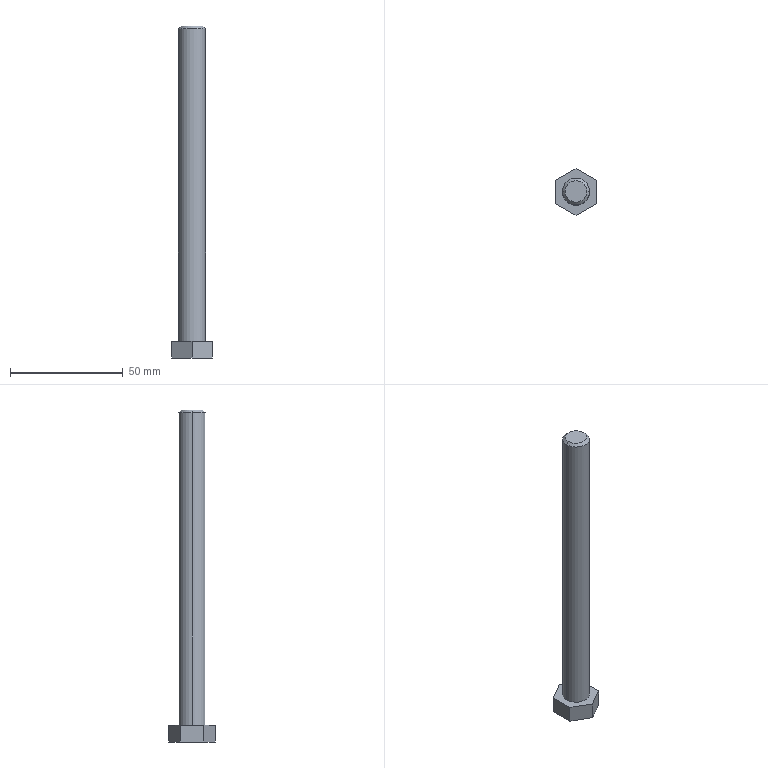Part | SolidWorks | features Chamfer 1, Extrusion 1, ICE 1, RefAxis 1 | 1 solid | 13 faces | box 18 x 20.785 x 147.5 mm | volume 17913 mm3 | plane 9 | cone 2 | cylinder 2 | commonest cylinder face diameters 12 x2
STEP:
#1=CARTESIAN_POINT('',(4.8,0.,147.5));
#2=VERTEX_POINT('',#1);
#3=CARTESIAN_POINT('',(-4.8,0.,147.5));
#4=VERTEX_POINT('',#3);
#5=CARTESIAN_POINT('',(0.,0.,147.5));
#6=DIRECTION('',(0.,0.,1.));
#7=DIRECTION('',(1.,0.,0.));
#8=AXIS2_PLACEMENT_3D('',#5,#6,#7);
#9=CIRCLE('',#8,4.8);
#10=EDGE_CURVE('',#2,#4,#9,.T.);
#11=ORIENTED_EDGE('',*,*,#10,.F.);
#12=CARTESIAN_POINT('',(6.,0.,146.3));
#13=VERTEX_POINT('',#12);
#14=CARTESIAN_POINT('',(4.8,0.,147.5));
#15=DIRECTION('',(0.7071,0.,-0.7071));
#16=VECTOR('',#15,1000.);
#17=LINE('',#14,#16);
#18=EDGE_CURVE('',#2,#13,#17,.T.);
#19=ORIENTED_EDGE('',*,*,#18,.T.);
#20=CARTESIAN_POINT('',(-6.,0.,146.3));
#21=VERTEX_POINT('',#20);
#22=CARTESIAN_POINT('',(0.,0.,146.3));
#23=DIRECTION('',(0.,0.,-1.));
#24=DIRECTION('',(1.,0.,0.));
#25=AXIS2_PLACEMENT_3D('',#22,#23,#24);
#26=CIRCLE('',#25,6.);
#27=EDGE_CURVE('',#21,#13,#26,.T.);
#28=ORIENTED_EDGE('',*,*,#27,.F.);
#29=CARTESIAN_POINT('',(-4.8,0.,147.5));
#30=DIRECTION('',(-0.7071,0.,-0.7071));
#31=VECTOR('',#30,1000.);
#32=LINE('',#29,#31);
#33=EDGE_CURVE('',#4,#21,#32,.T.);
#34=ORIENTED_EDGE('',*,*,#33,.F.);
#35=EDGE_LOOP('',(#11,#19,#28,#34));
#36=FACE_OUTER_BOUND('',#35,.T.);
#37=CARTESIAN_POINT('',(0.,0.,147.5));
#38=DIRECTION('',(0.,0.,-1.));
#39=DIRECTION('',(-1.,0.,0.));
#40=AXIS2_PLACEMENT_3D('',#37,#38,#39);
#41=CONICAL_SURFACE('',#40,4.8,0.7854);
#42=ADVANCED_FACE('',(#36),#41,.T.);
#43=ORIENTED_EDGE('',*,*,#27,.T.);
#44=CARTESIAN_POINT('',(6.,0.,7.5));
#45=VERTEX_POINT('',#44);
#46=CARTESIAN_POINT('',(6.,0.,147.5));
#47=DIRECTION('',(0.,0.,-1.));
#48=VECTOR('',#47,1000.);
#49=LINE('',#46,#48);
#50=EDGE_CURVE('',#13,#45,#49,.T.);
#51=ORIENTED_EDGE('',*,*,#50,.T.);
#52=CARTESIAN_POINT('',(-6.,0.,7.5));
#53=VERTEX_POINT('',#52);
#54=CARTESIAN_POINT('',(0.,0.,7.5));
#55=DIRECTION('',(0.,0.,1.));
#56=DIRECTION('',(1.,0.,0.));
#57=AXIS2_PLACEMENT_3D('',#54,#55,#56);
#58=CIRCLE('',#57,6.);
#59=EDGE_CURVE('',#45,#53,#58,.T.);
#60=ORIENTED_EDGE('',*,*,#59,.T.);
#61=CARTESIAN_POINT('',(-6.,0.,147.5));
#62=DIRECTION('',(0.,0.,-1.));
#63=VECTOR('',#62,1000.);
#64=LINE('',#61,#63);
#65=EDGE_CURVE('',#21,#53,#64,.T.);
#66=ORIENTED_EDGE('',*,*,#65,.F.);
#67=EDGE_LOOP('',(#43,#51,#60,#66));
#68=FACE_OUTER_BOUND('',#67,.T.);
#69=CARTESIAN_POINT('',(0.,0.,147.5));
#70=DIRECTION('',(0.,0.,-1.));
#71=DIRECTION('',(-1.,0.,0.));
#72=AXIS2_PLACEMENT_3D('',#69,#70,#71);
#73=CYLINDRICAL_SURFACE('',#72,6.);
#74=ADVANCED_FACE('',(#68),#73,.T.);
#75=CARTESIAN_POINT('',(9.,-5.196,7.5));
#76=VERTEX_POINT('',#75);
#77=CARTESIAN_POINT('',(9.,5.196,7.5));
#78=VERTEX_POINT('',#77);
#79=CARTESIAN_POINT('',(9.,-5.196,7.5));
#80=DIRECTION('',(0.,1.,0.));
#81=VECTOR('',#80,1000.);
#82=LINE('',#79,#81);
#83=EDGE_CURVE('',#76,#78,#82,.T.);
#84=ORIENTED_EDGE('',*,*,#83,.T.);
#85=CARTESIAN_POINT('',(0.,10.392,7.5));
#86=VERTEX_POINT('',#85);
#87=CARTESIAN_POINT('',(9.,5.196,7.5));
#88=DIRECTION('',(-0.866,0.5,0.));
#89=VECTOR('',#88,1000.);
#90=LINE('',#87,#89);
#91=EDGE_CURVE('',#78,#86,#90,.T.);
#92=ORIENTED_EDGE('',*,*,#91,.T.);
#93=CARTESIAN_POINT('',(-9.,5.196,7.5));
#94=VERTEX_POINT('',#93);
#95=CARTESIAN_POINT('',(0.,10.392,7.5));
#96=DIRECTION('',(-0.866,-0.5,0.));
#97=VECTOR('',#96,1000.);
#98=LINE('',#95,#97);
#99=EDGE_CURVE('',#86,#94,#98,.T.);
#100=ORIENTED_EDGE('',*,*,#99,.T.);
#101=CARTESIAN_POINT('',(-9.,-5.196,7.5));
#102=VERTEX_POINT('',#101);
#103=CARTESIAN_POINT('',(-9.,5.196,7.5));
#104=DIRECTION('',(0.,-1.,0.));
#105=VECTOR('',#104,1000.);
#106=LINE('',#103,#105);
#107=EDGE_CURVE('',#94,#102,#106,.T.);
#108=ORIENTED_EDGE('',*,*,#107,.T.);
#109=CARTESIAN_POINT('',(0.,-10.392,7.5));
#110=VERTEX_POINT('',#109);
#111=CARTESIAN_POINT('',(-9.,-5.196,7.5));
#112=DIRECTION('',(0.866,-0.5,0.));
#113=VECTOR('',#112,1000.);
#114=LINE('',#111,#113);
#115=EDGE_CURVE('',#102,#110,#114,.T.);
#116=ORIENTED_EDGE('',*,*,#115,.T.);
#117=CARTESIAN_POINT('',(0.,-10.392,7.5));
#118=DIRECTION('',(0.866,0.5,0.));
#119=VECTOR('',#118,1000.);
#120=LINE('',#117,#119);
#121=EDGE_CURVE('',#110,#76,#120,.T.);
#122=ORIENTED_EDGE('',*,*,#121,.T.);
#123=EDGE_LOOP('',(#84,#92,#100,#108,#116,#122));
#124=FACE_OUTER_BOUND('',#123,.T.);
#125=CARTESIAN_POINT('',(0.,0.,7.5));
#126=DIRECTION('',(0.,0.,1.));
#127=DIRECTION('',(1.,0.,0.));
#128=AXIS2_PLACEMENT_3D('',#125,#126,#127);
#129=CIRCLE('',#128,6.);
#130=EDGE_CURVE('',#53,#45,#129,.T.);
#131=ORIENTED_EDGE('',*,*,#130,.F.);
#132=ORIENTED_EDGE('',*,*,#59,.F.);
#133=EDGE_LOOP('',(#131,#132));
#134=FACE_BOUND('',#133,.T.);
#135=CARTESIAN_POINT('',(0.,0.,7.5));
#136=DIRECTION('',(0.,0.,1.));
#137=DIRECTION('',(1.,0.,0.));
#138=AXIS2_PLACEMENT_3D('',#135,#136,#137);
#139=PLANE('',#138);
#140=ADVANCED_FACE('',(#124,#134),#139,.T.);
#141=CARTESIAN_POINT('',(9.,-5.196,0.));
#142=VERTEX_POINT('',#141);
#143=CARTESIAN_POINT('',(9.,5.196,0.));
#144=VERTEX_POINT('',#143);
#145=CARTESIAN_POINT('',(9.,-5.196,0.));
#146=DIRECTION('',(0.,1.,0.));
#147=VECTOR('',#146,1000.);
#148=LINE('',#145,#147);
#149=EDGE_CURVE('',#142,#144,#148,.T.);
#150=ORIENTED_EDGE('',*,*,#149,.T.);
#151=CARTESIAN_POINT('',(9.,5.196,7.5));
#152=DIRECTION('',(0.,0.,-1.));
#153=VECTOR('',#152,1000.);
#154=LINE('',#151,#153);
#155=EDGE_CURVE('',#78,#144,#154,.T.);
#156=ORIENTED_EDGE('',*,*,#155,.F.);
#157=ORIENTED_EDGE('',*,*,#83,.F.);
#158=CARTESIAN_POINT('',(9.,-5.196,7.5));
#159=DIRECTION('',(0.,0.,-1.));
#160=VECTOR('',#159,1000.);
#161=LINE('',#158,#160);
#162=EDGE_CURVE('',#76,#142,#161,.T.);
#163=ORIENTED_EDGE('',*,*,#162,.T.);
#164=EDGE_LOOP('',(#150,#156,#157,#163));
#165=FACE_OUTER_BOUND('',#164,.T.);
#166=CARTESIAN_POINT('',(9.,-5.196,7.5));
#167=DIRECTION('',(-1.,0.,0.));
#168=DIRECTION('',(0.,-1.,0.));
#169=AXIS2_PLACEMENT_3D('',#166,#167,#168);
#170=PLANE('',#169);
#171=ADVANCED_FACE('',(#165),#170,.F.);
#172=CARTESIAN_POINT('',(0.,10.392,0.));
#173=VERTEX_POINT('',#172);
#174=CARTESIAN_POINT('',(9.,5.196,0.));
#175=DIRECTION('',(-0.866,0.5,0.));
#176=VECTOR('',#175,1000.);
#177=LINE('',#174,#176);
#178=EDGE_CURVE('',#144,#173,#177,.T.);
#179=ORIENTED_EDGE('',*,*,#178,.T.);
#180=CARTESIAN_POINT('',(0.,10.392,7.5));
#181=DIRECTION('',(0.,0.,-1.));
#182=VECTOR('',#181,1000.);
#183=LINE('',#180,#182);
#184=EDGE_CURVE('',#86,#173,#183,.T.);
#185=ORIENTED_EDGE('',*,*,#184,.F.);
#186=ORIENTED_EDGE('',*,*,#91,.F.);
#187=ORIENTED_EDGE('',*,*,#155,.T.);
#188=EDGE_LOOP('',(#179,#185,#186,#187));
#189=FACE_OUTER_BOUND('',#188,.T.);
#190=CARTESIAN_POINT('',(9.,5.196,7.5));
#191=DIRECTION('',(-0.5,-0.866,0.));
#192=DIRECTION('',(0.866,-0.5,0.));
#193=AXIS2_PLACEMENT_3D('',#190,#191,#192);
#194=PLANE('',#193);
#195=ADVANCED_FACE('',(#189),#194,.F.);
#196=CARTESIAN_POINT('',(-9.,5.196,0.));
#197=VERTEX_POINT('',#196);
#198=CARTESIAN_POINT('',(0.,10.392,0.));
#199=DIRECTION('',(-0.866,-0.5,0.));
#200=VECTOR('',#199,1000.);
#201=LINE('',#198,#200);
#202=EDGE_CURVE('',#173,#197,#201,.T.);
#203=ORIENTED_EDGE('',*,*,#202,.T.);
#204=CARTESIAN_POINT('',(-9.,5.196,7.5));
#205=DIRECTION('',(0.,0.,-1.));
#206=VECTOR('',#205,1000.);
#207=LINE('',#204,#206);
#208=EDGE_CURVE('',#94,#197,#207,.T.);
#209=ORIENTED_EDGE('',*,*,#208,.F.);
#210=ORIENTED_EDGE('',*,*,#99,.F.);
#211=ORIENTED_EDGE('',*,*,#184,.T.);
#212=EDGE_LOOP('',(#203,#209,#210,#211));
#213=FACE_OUTER_BOUND('',#212,.T.);
#214=CARTESIAN_POINT('',(0.,10.392,7.5));
#215=DIRECTION('',(0.5,-0.866,0.));
#216=DIRECTION('',(0.866,0.5,0.));
#217=AXIS2_PLACEMENT_3D('',#214,#215,#216);
#218=PLANE('',#217);
#219=ADVANCED_FACE('',(#213),#218,.F.);
#220=CARTESIAN_POINT('',(-9.,-5.196,0.));
#221=VERTEX_POINT('',#220);
#222=CARTESIAN_POINT('',(-9.,5.196,0.));
#223=DIRECTION('',(0.,-1.,0.));
#224=VECTOR('',#223,1000.);
#225=LINE('',#222,#224);
#226=EDGE_CURVE('',#197,#221,#225,.T.);
#227=ORIENTED_EDGE('',*,*,#226,.T.);
#228=CARTESIAN_POINT('',(-9.,-5.196,7.5));
#229=DIRECTION('',(0.,0.,-1.));
#230=VECTOR('',#229,1000.);
#231=LINE('',#228,#230);
#232=EDGE_CURVE('',#102,#221,#231,.T.);
#233=ORIENTED_EDGE('',*,*,#232,.F.);
#234=ORIENTED_EDGE('',*,*,#107,.F.);
#235=ORIENTED_EDGE('',*,*,#208,.T.);
#236=EDGE_LOOP('',(#227,#233,#234,#235));
#237=FACE_OUTER_BOUND('',#236,.T.);
#238=CARTESIAN_POINT('',(-9.,5.196,7.5));
#239=DIRECTION('',(1.,0.,0.));
#240=DIRECTION('',(0.,0.,-1.));
#241=AXIS2_PLACEMENT_3D('',#238,#239,#240);
#242=PLANE('',#241);
#243=ADVANCED_FACE('',(#237),#242,.F.);
#244=CARTESIAN_POINT('',(0.,-10.392,0.));
#245=VERTEX_POINT('',#244);
#246=CARTESIAN_POINT('',(-9.,-5.196,0.));
#247=DIRECTION('',(0.866,-0.5,0.));
#248=VECTOR('',#247,1000.);
#249=LINE('',#246,#248);
#250=EDGE_CURVE('',#221,#245,#249,.T.);
#251=ORIENTED_EDGE('',*,*,#250,.T.);
#252=CARTESIAN_POINT('',(0.,-10.392,7.5));
#253=DIRECTION('',(0.,0.,-1.));
#254=VECTOR('',#253,1000.);
#255=LINE('',#252,#254);
#256=EDGE_CURVE('',#110,#245,#255,.T.);
#257=ORIENTED_EDGE('',*,*,#256,.F.);
#258=ORIENTED_EDGE('',*,*,#115,.F.);
#259=ORIENTED_EDGE('',*,*,#232,.T.);
#260=EDGE_LOOP('',(#251,#257,#258,#259));
#261=FACE_OUTER_BOUND('',#260,.T.);
#262=CARTESIAN_POINT('',(-9.,-5.196,7.5));
#263=DIRECTION('',(0.5,0.866,0.));
#264=DIRECTION('',(-0.866,0.5,0.));
#265=AXIS2_PLACEMENT_3D('',#262,#263,#264);
#266=PLANE('',#265);
#267=ADVANCED_FACE('',(#261),#266,.F.);
#268=CARTESIAN_POINT('',(0.,-10.392,0.));
#269=DIRECTION('',(0.866,0.5,0.));
#270=VECTOR('',#269,1000.);
#271=LINE('',#268,#270);
#272=EDGE_CURVE('',#245,#142,#271,.T.);
#273=ORIENTED_EDGE('',*,*,#272,.T.);
#274=ORIENTED_EDGE('',*,*,#162,.F.);
#275=ORIENTED_EDGE('',*,*,#121,.F.);
#276=ORIENTED_EDGE('',*,*,#256,.T.);
#277=EDGE_LOOP('',(#273,#274,#275,#276));
#278=FACE_OUTER_BOUND('',#277,.T.);
#279=CARTESIAN_POINT('',(0.,-10.392,7.5));
#280=DIRECTION('',(-0.5,0.866,0.));
#281=DIRECTION('',(-0.866,-0.5,0.));
#282=AXIS2_PLACEMENT_3D('',#279,#280,#281);
#283=PLANE('',#282);
#284=ADVANCED_FACE('',(#278),#283,.F.);
#285=ORIENTED_EDGE('',*,*,#149,.F.);
#286=ORIENTED_EDGE('',*,*,#272,.F.);
#287=ORIENTED_EDGE('',*,*,#250,.F.);
#288=ORIENTED_EDGE('',*,*,#226,.F.);
#289=ORIENTED_EDGE('',*,*,#202,.F.);
#290=ORIENTED_EDGE('',*,*,#178,.F.);
#291=EDGE_LOOP('',(#285,#286,#287,#288,#289,#290));
#292=FACE_OUTER_BOUND('',#291,.T.);
#293=CARTESIAN_POINT('',(0.,0.,0.));
#294=DIRECTION('',(0.,0.,1.));
#295=DIRECTION('',(1.,0.,0.));
#296=AXIS2_PLACEMENT_3D('',#293,#294,#295);
#297=PLANE('',#296);
#298=ADVANCED_FACE('',(#292),#297,.F.);
#299=ORIENTED_EDGE('',*,*,#50,.F.);
#300=CARTESIAN_POINT('',(0.,0.,146.3));
#301=DIRECTION('',(0.,0.,-1.));
#302=DIRECTION('',(1.,0.,0.));
#303=AXIS2_PLACEMENT_3D('',#300,#301,#302);
#304=CIRCLE('',#303,6.);
#305=EDGE_CURVE('',#13,#21,#304,.T.);
#306=ORIENTED_EDGE('',*,*,#305,.T.);
#307=ORIENTED_EDGE('',*,*,#65,.T.);
#308=ORIENTED_EDGE('',*,*,#130,.T.);
#309=EDGE_LOOP('',(#299,#306,#307,#308));
#310=FACE_OUTER_BOUND('',#309,.T.);
#311=CARTESIAN_POINT('',(0.,0.,147.5));
#312=DIRECTION('',(0.,0.,-1.));
#313=DIRECTION('',(-1.,0.,0.));
#314=AXIS2_PLACEMENT_3D('',#311,#312,#313);
#315=CYLINDRICAL_SURFACE('',#314,6.);
#316=ADVANCED_FACE('',(#310),#315,.T.);
#317=CARTESIAN_POINT('',(0.,0.,147.5));
#318=DIRECTION('',(0.,0.,1.));
#319=DIRECTION('',(1.,0.,0.));
#320=AXIS2_PLACEMENT_3D('',#317,#318,#319);
#321=CIRCLE('',#320,4.8);
#322=EDGE_CURVE('',#4,#2,#321,.T.);
#323=ORIENTED_EDGE('',*,*,#322,.T.);
#324=ORIENTED_EDGE('',*,*,#10,.T.);
#325=EDGE_LOOP('',(#323,#324));
#326=FACE_OUTER_BOUND('',#325,.T.);
#327=CARTESIAN_POINT('',(0.,0.,147.5));
#328=DIRECTION('',(0.,0.,1.));
#329=DIRECTION('',(1.,0.,0.));
#330=AXIS2_PLACEMENT_3D('',#327,#328,#329);
#331=PLANE('',#330);
#332=ADVANCED_FACE('',(#326),#331,.T.);
#333=ORIENTED_EDGE('',*,*,#18,.F.);
#334=ORIENTED_EDGE('',*,*,#322,.F.);
#335=ORIENTED_EDGE('',*,*,#33,.T.);
#336=ORIENTED_EDGE('',*,*,#305,.F.);
#337=EDGE_LOOP('',(#333,#334,#335,#336));
#338=FACE_OUTER_BOUND('',#337,.T.);
#339=CARTESIAN_POINT('',(0.,0.,147.5));
#340=DIRECTION('',(0.,0.,-1.));
#341=DIRECTION('',(-1.,0.,0.));
#342=AXIS2_PLACEMENT_3D('',#339,#340,#341);
#343=CONICAL_SURFACE('',#342,4.8,0.7854);
#344=ADVANCED_FACE('',(#338),#343,.T.);
#345=CLOSED_SHELL('',(#42,#74,#140,#171,#195,#219,#243,#267,#284,#298,#316,#332,#344));
#346=MANIFOLD_SOLID_BREP('',#345);
#347=CARTESIAN_POINT('',(0.,0.,0.));
#348=DIRECTION('',(0.,0.,1.));
#349=DIRECTION('',(1.,0.,0.));
#350=AXIS2_PLACEMENT_3D('',#347,#348,#349);
#351=(LENGTH_UNIT()NAMED_UNIT(*)SI_UNIT(.MILLI.,.METRE.));
#352=UNCERTAINTY_MEASURE_WITH_UNIT(LENGTH_MEASURE(0.00001),#351,'','');
#353=(NAMED_UNIT(*)PLANE_ANGLE_UNIT()SI_UNIT($,.RADIAN.));
#354=(NAMED_UNIT(*)SI_UNIT($,.STERADIAN.)SOLID_ANGLE_UNIT());
#355=(GEOMETRIC_REPRESENTATION_CONTEXT(3)GLOBAL_UNCERTAINTY_ASSIGNED_CONTEXT((#352))GLOBAL_UNIT_ASSIGNED_CONTEXT((#351,#353,#354))REPRESENTATION_CONTEXT('',''));
#356=ADVANCED_BREP_SHAPE_REPRESENTATION('',(#346,#350),#355);